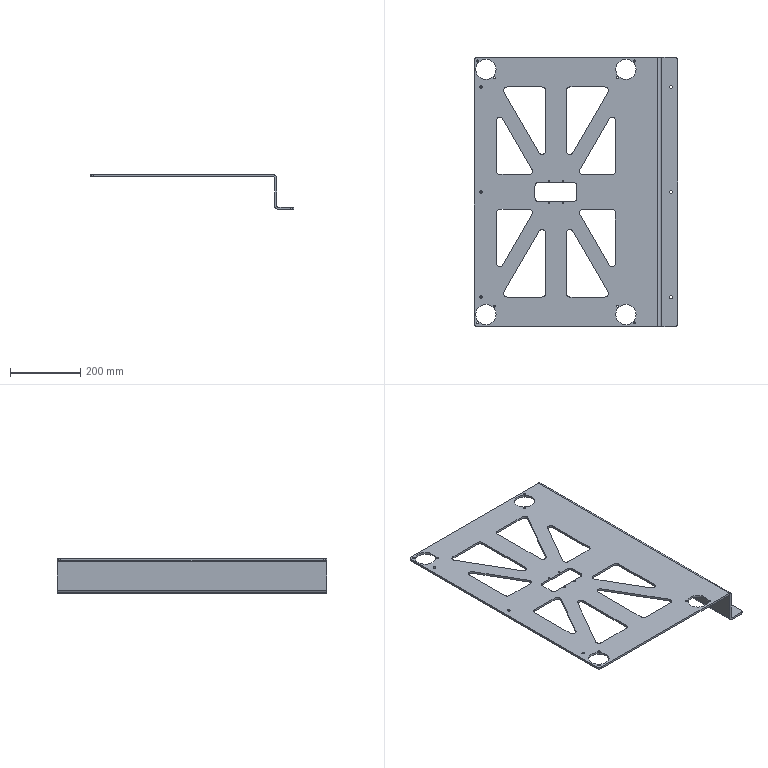Part | STEP file | LOWER.BRACKET.stp | 1 solid | 128 faces | box 582.5 x 770 x 98 mm | volume 2415812 mm3 | cylinder 62 | spline 43 | plane 23 | commonest cylinder face diameters 20 x26 6 x12 7 x6 8 x6 5 x4 18 x4